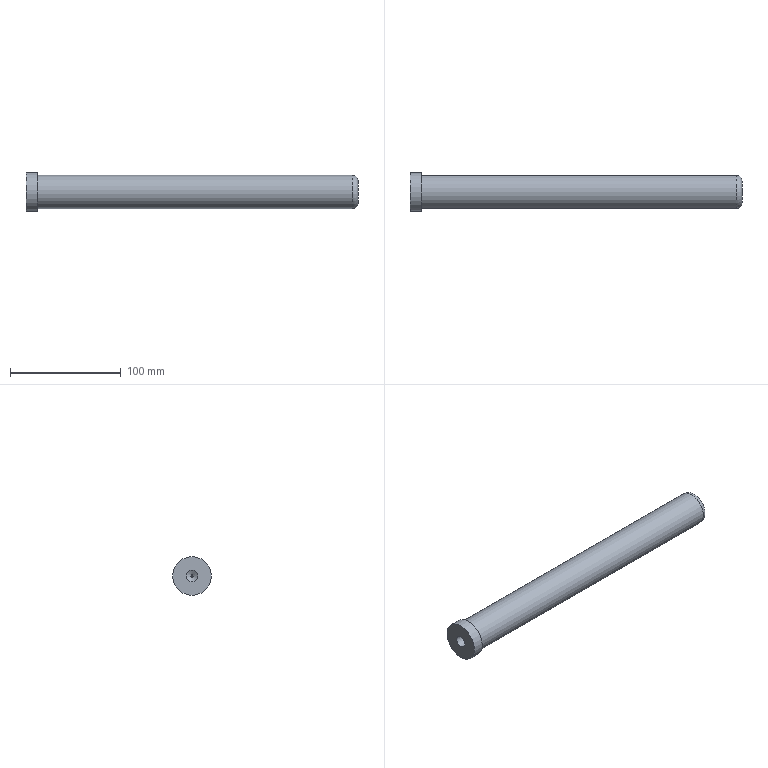Part | STEP file | solid 73 | 1 solid | 9 faces | box 300 x 35 x 35 mm | volume 211977 mm3 | plane 4 | cylinder 3 | cone 1 | torus 1 | commonest cylinder face diameters 10.5 x1 30 x1 35 x1